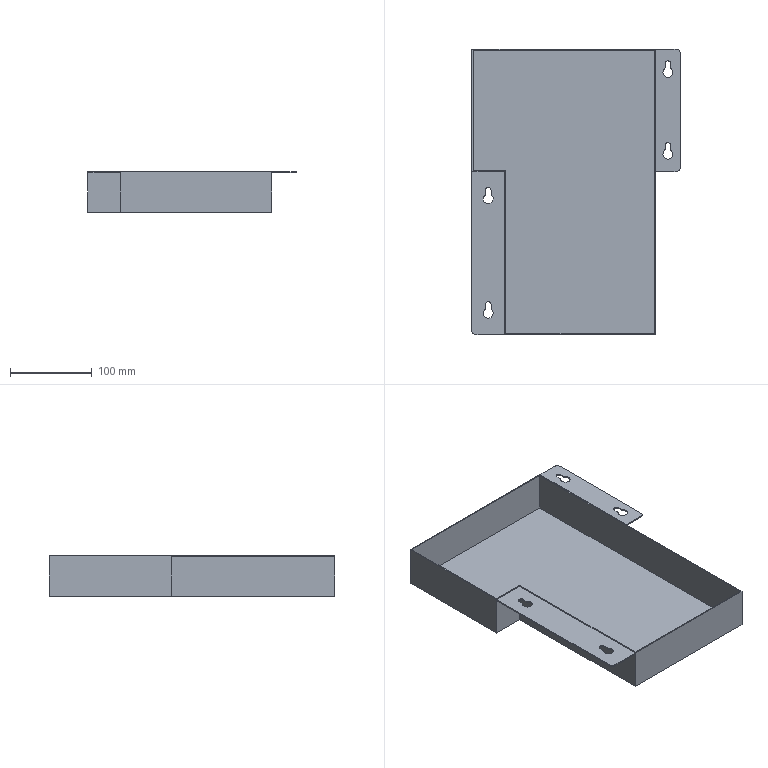Part | SolidWorks | features Fillet 2, ICE 2, Cut 1, Extrusion 1, Shell 1 | 3 solids | 62 faces | box 255 x 350 x 50 mm | volume 207064 mm3 | plane 35 | cylinder 27 | commonest cylinder face diameters 12 x12 4 x8 7 x4 10 x3